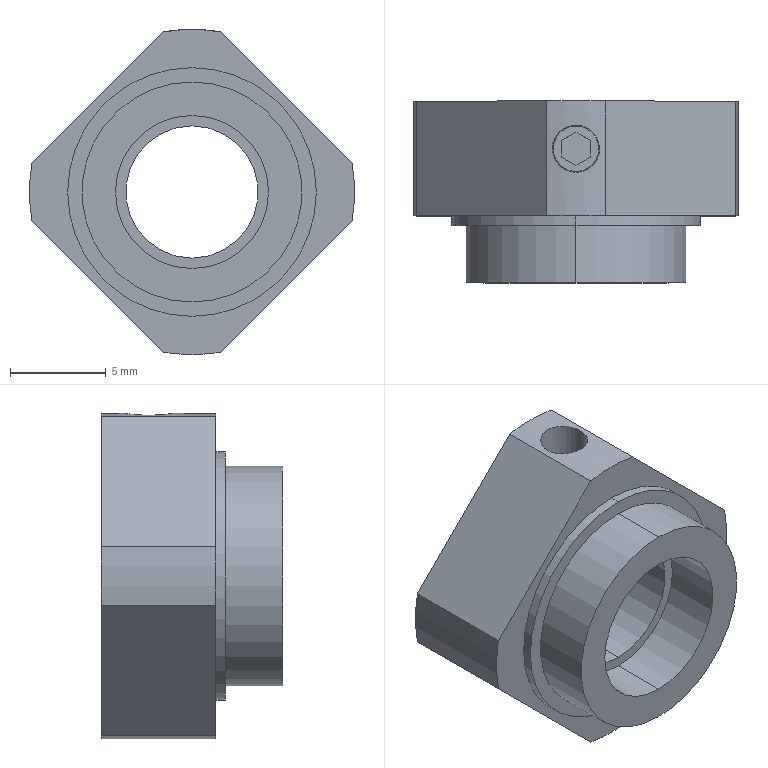Part | SolidWorks | features BaseBody 1 | 1 solid | 41 faces | box 17 x 9.5 x 17 mm | volume 1093 mm3 | plane 18 | cylinder 17 | cone 6 | commonest cylinder face diameters 17 x5 2.459 x4 6.917 x2 8 x2 11.5 x2 13 x2
STEP:
#1=CARTESIAN_POINT('',(290.547,1682.923,-1182.029));
#2=VERTEX_POINT('',#1);
#3=CARTESIAN_POINT('',(290.547,1682.923,-1175.111));
#4=VERTEX_POINT('',#3);
#5=CARTESIAN_POINT('',(290.547,1682.923,-1178.57));
#6=DIRECTION('',(0.,1.,0.));
#7=DIRECTION('',(0.,0.,-1.));
#8=AXIS2_PLACEMENT_3D('',#5,#6,#7);
#9=CIRCLE('',#8,3.459);
#10=EDGE_CURVE('',#2,#4,#9,.T.);
#11=ORIENTED_EDGE('',*,*,#10,.F.);
#12=CARTESIAN_POINT('',(290.547,1683.464,-1182.57));
#13=VERTEX_POINT('',#12);
#14=CARTESIAN_POINT('',(290.547,1683.464,-1182.57));
#15=DIRECTION('',(0.,0.7071,-0.7071));
#16=VECTOR('',#15,1000.);
#17=LINE('',#14,#16);
#18=EDGE_CURVE('',#2,#13,#17,.T.);
#19=ORIENTED_EDGE('',*,*,#18,.T.);
#20=CARTESIAN_POINT('',(290.547,1683.464,-1174.57));
#21=VERTEX_POINT('',#20);
#22=CARTESIAN_POINT('',(290.547,1683.464,-1178.57));
#23=DIRECTION('',(0.,-1.,0.));
#24=DIRECTION('',(0.,0.,1.));
#25=AXIS2_PLACEMENT_3D('',#22,#23,#24);
#26=CIRCLE('',#25,4.);
#27=EDGE_CURVE('',#21,#13,#26,.T.);
#28=ORIENTED_EDGE('',*,*,#27,.F.);
#29=CARTESIAN_POINT('',(290.547,1683.464,-1174.57));
#30=DIRECTION('',(0.,0.7071,0.7071));
#31=VECTOR('',#30,1000.);
#32=LINE('',#29,#31);
#33=EDGE_CURVE('',#4,#21,#32,.T.);
#34=ORIENTED_EDGE('',*,*,#33,.F.);
#35=EDGE_LOOP('',(#11,#19,#28,#34));
#36=FACE_OUTER_BOUND('',#35,.T.);
#37=CARTESIAN_POINT('',(290.547,1683.464,-1178.57));
#38=DIRECTION('',(0.,1.,0.));
#39=DIRECTION('',(0.,0.,1.));
#40=AXIS2_PLACEMENT_3D('',#37,#38,#39);
#41=CONICAL_SURFACE('',#40,4.,0.7854);
#42=ADVANCED_FACE('',(#36),#41,.F.);
#43=CARTESIAN_POINT('',(290.547,1683.464,-1187.07));
#44=VERTEX_POINT('',#43);
#45=CARTESIAN_POINT('',(289.006,1683.464,-1186.929));
#46=VERTEX_POINT('',#45);
#47=CARTESIAN_POINT('',(290.547,1683.464,-1178.57));
#48=DIRECTION('',(0.,1.,0.));
#49=DIRECTION('',(0.,0.,-1.));
#50=AXIS2_PLACEMENT_3D('',#47,#48,#49);
#51=CIRCLE('',#50,8.5);
#52=EDGE_CURVE('',#44,#46,#51,.T.);
#53=ORIENTED_EDGE('',*,*,#52,.F.);
#54=CARTESIAN_POINT('',(290.547,1677.464,-1187.07));
#55=VERTEX_POINT('',#54);
#56=CARTESIAN_POINT('',(290.547,1654.964,-1187.07));
#57=DIRECTION('',(0.,-1.,0.));
#58=VECTOR('',#57,1000.);
#59=LINE('',#56,#58);
#60=EDGE_CURVE('',#44,#55,#59,.T.);
#61=ORIENTED_EDGE('',*,*,#60,.T.);
#62=CARTESIAN_POINT('',(289.006,1677.464,-1186.929));
#63=VERTEX_POINT('',#62);
#64=CARTESIAN_POINT('',(290.547,1677.464,-1178.57));
#65=DIRECTION('',(0.,1.,0.));
#66=DIRECTION('',(0.,0.,-1.));
#67=AXIS2_PLACEMENT_3D('',#64,#65,#66);
#68=CIRCLE('',#67,8.5);
#69=EDGE_CURVE('',#55,#63,#68,.T.);
#70=ORIENTED_EDGE('',*,*,#69,.T.);
#71=CARTESIAN_POINT('',(289.006,1683.464,-1186.929));
#72=DIRECTION('',(0.,1.,0.));
#73=VECTOR('',#72,1000.);
#74=LINE('',#71,#73);
#75=EDGE_CURVE('',#63,#46,#74,.T.);
#76=ORIENTED_EDGE('',*,*,#75,.T.);
#77=EDGE_LOOP('',(#53,#61,#70,#76));
#78=FACE_OUTER_BOUND('',#77,.T.);
#79=CARTESIAN_POINT('',(290.547,1654.964,-1178.57));
#80=DIRECTION('',(0.,-1.,0.));
#81=DIRECTION('',(0.,0.,-1.));
#82=AXIS2_PLACEMENT_3D('',#79,#80,#81);
#83=CYLINDRICAL_SURFACE('',#82,8.5);
#84=ADVANCED_FACE('',(#78),#83,.T.);
#85=ORIENTED_EDGE('',*,*,#10,.T.);
#86=CARTESIAN_POINT('',(290.547,1682.194,-1175.111));
#87=VERTEX_POINT('',#86);
#88=CARTESIAN_POINT('',(290.547,1654.964,-1175.111));
#89=DIRECTION('',(0.,-1.,0.));
#90=VECTOR('',#89,1000.);
#91=LINE('',#88,#90);
#92=EDGE_CURVE('',#4,#87,#91,.T.);
#93=ORIENTED_EDGE('',*,*,#92,.T.);
#94=CARTESIAN_POINT('',(289.317,1680.964,-1175.337));
#95=VERTEX_POINT('',#94);
#96=CARTESIAN_POINT('',(289.317,1680.964,-1175.337));
#97=CARTESIAN_POINT('',(289.317,1681.128,-1175.337));
#98=CARTESIAN_POINT('',(289.35,1681.288,-1175.325));
#99=CARTESIAN_POINT('',(289.473,1681.585,-1175.282));
#100=CARTESIAN_POINT('',(289.565,1681.721,-1175.252));
#101=CARTESIAN_POINT('',(289.789,1681.945,-1175.193));
#102=CARTESIAN_POINT('',(289.925,1682.037,-1175.165));
#103=CARTESIAN_POINT('',(290.22,1682.16,-1175.124));
#104=CARTESIAN_POINT('',(290.383,1682.194,-1175.111));
#105=CARTESIAN_POINT('',(290.547,1682.194,-1175.111));
#106=B_SPLINE_CURVE_WITH_KNOTS('',3,(#96,#97,#98,#99,#100,#101,#102,#103,#104,#105),.UNSPECIFIED.,.F.,.F.,(4,2,2,2,4),(0.001937,0.002421,0.002905,0.003389,0.003874),.UNSPECIFIED.);
#107=EDGE_CURVE('',#95,#87,#106,.T.);
#108=ORIENTED_EDGE('',*,*,#107,.F.);
#109=CARTESIAN_POINT('',(290.547,1679.735,-1175.111));
#110=VERTEX_POINT('',#109);
#111=CARTESIAN_POINT('',(290.547,1679.735,-1175.111));
#112=CARTESIAN_POINT('',(290.383,1679.735,-1175.111));
#113=CARTESIAN_POINT('',(290.222,1679.767,-1175.123));
#114=CARTESIAN_POINT('',(289.925,1679.891,-1175.165));
#115=CARTESIAN_POINT('',(289.789,1679.982,-1175.193));
#116=CARTESIAN_POINT('',(289.565,1680.207,-1175.252));
#117=CARTESIAN_POINT('',(289.474,1680.343,-1175.282));
#118=CARTESIAN_POINT('',(289.35,1680.638,-1175.324));
#119=CARTESIAN_POINT('',(289.317,1680.8,-1175.337));
#120=CARTESIAN_POINT('',(289.317,1680.964,-1175.337));
#121=B_SPLINE_CURVE_WITH_KNOTS('',3,(#111,#112,#113,#114,#115,#116,#117,#118,#119,#120),.UNSPECIFIED.,.F.,.F.,(4,2,2,2,4),(0.000000144,0.0004843,0.0009685,0.001453,0.001937),.UNSPECIFIED.);
#122=EDGE_CURVE('',#110,#95,#121,.T.);
#123=ORIENTED_EDGE('',*,*,#122,.F.);
#124=CARTESIAN_POINT('',(290.547,1676.964,-1175.111));
#125=VERTEX_POINT('',#124);
#126=CARTESIAN_POINT('',(290.547,1654.964,-1175.111));
#127=DIRECTION('',(0.,-1.,0.));
#128=VECTOR('',#127,1000.);
#129=LINE('',#126,#128);
#130=EDGE_CURVE('',#110,#125,#129,.T.);
#131=ORIENTED_EDGE('',*,*,#130,.T.);
#132=CARTESIAN_POINT('',(290.547,1676.964,-1182.028));
#133=VERTEX_POINT('',#132);
#134=CARTESIAN_POINT('',(290.547,1676.964,-1178.57));
#135=DIRECTION('',(0.,1.,0.));
#136=DIRECTION('',(0.,0.,-1.));
#137=AXIS2_PLACEMENT_3D('',#134,#135,#136);
#138=CIRCLE('',#137,3.459);
#139=EDGE_CURVE('',#133,#125,#138,.T.);
#140=ORIENTED_EDGE('',*,*,#139,.F.);
#141=CARTESIAN_POINT('',(290.547,1654.964,-1182.028));
#142=DIRECTION('',(0.,-1.,0.));
#143=VECTOR('',#142,1000.);
#144=LINE('',#141,#143);
#145=EDGE_CURVE('',#2,#133,#144,.T.);
#146=ORIENTED_EDGE('',*,*,#145,.F.);
#147=EDGE_LOOP('',(#85,#93,#108,#123,#131,#140,#146));
#148=FACE_OUTER_BOUND('',#147,.T.);
#149=CARTESIAN_POINT('',(290.547,1654.964,-1178.57));
#150=DIRECTION('',(0.,-1.,0.));
#151=DIRECTION('',(0.,0.,-1.));
#152=AXIS2_PLACEMENT_3D('',#149,#150,#151);
#153=CYLINDRICAL_SURFACE('',#152,3.459);
#154=ADVANCED_FACE('',(#148),#153,.F.);
#155=CARTESIAN_POINT('',(289.317,1680.964,-1172.132));
#156=VERTEX_POINT('',#155);
#157=CARTESIAN_POINT('',(291.776,1680.964,-1172.132));
#158=VERTEX_POINT('',#157);
#159=CARTESIAN_POINT('',(290.547,1680.964,-1172.132));
#160=DIRECTION('',(0.,0.,1.));
#161=DIRECTION('',(1.,0.,0.));
#162=AXIS2_PLACEMENT_3D('',#159,#160,#161);
#163=CIRCLE('',#162,1.229);
#164=EDGE_CURVE('',#156,#158,#163,.T.);
#165=ORIENTED_EDGE('',*,*,#164,.F.);
#166=CARTESIAN_POINT('',(289.317,1680.964,-1170.159));
#167=VERTEX_POINT('',#166);
#168=CARTESIAN_POINT('',(289.317,1680.964,-1170.07));
#169=DIRECTION('',(0.,0.,1.));
#170=VECTOR('',#169,1000.);
#171=LINE('',#168,#170);
#172=EDGE_CURVE('',#156,#167,#171,.T.);
#173=ORIENTED_EDGE('',*,*,#172,.T.);
#174=CARTESIAN_POINT('',(291.776,1680.964,-1170.159));
#175=VERTEX_POINT('',#174);
#176=CARTESIAN_POINT('',(291.776,1680.964,-1170.159));
#177=CARTESIAN_POINT('',(291.776,1680.801,-1170.159));
#178=CARTESIAN_POINT('',(291.744,1680.642,-1170.155));
#179=CARTESIAN_POINT('',(291.621,1680.344,-1170.138));
#180=CARTESIAN_POINT('',(291.529,1680.208,-1170.126));
#181=CARTESIAN_POINT('',(291.303,1679.982,-1170.103));
#182=CARTESIAN_POINT('',(291.166,1679.89,-1170.091));
#183=CARTESIAN_POINT('',(290.871,1679.767,-1170.075));
#184=CARTESIAN_POINT('',(290.709,1679.735,-1170.07));
#185=CARTESIAN_POINT('',(290.384,1679.735,-1170.07));
#186=CARTESIAN_POINT('',(290.224,1679.767,-1170.075));
#187=CARTESIAN_POINT('',(289.927,1679.89,-1170.091));
#188=CARTESIAN_POINT('',(289.791,1679.981,-1170.103));
#189=CARTESIAN_POINT('',(289.564,1680.208,-1170.126));
#190=CARTESIAN_POINT('',(289.473,1680.344,-1170.138));
#191=CARTESIAN_POINT('',(289.35,1680.64,-1170.154));
#192=CARTESIAN_POINT('',(289.317,1680.801,-1170.159));
#193=CARTESIAN_POINT('',(289.317,1680.964,-1170.159));
#194=B_SPLINE_CURVE_WITH_KNOTS('',3,(#176,#177,#178,#179,#180,#181,#182,#183,#184,#185,#186,#187,#188,#189,#190,#191,#192,#193),.UNSPECIFIED.,.F.,.F.,(4,2,2,2,2,2,2,2,4),(-0.003846,-0.003366,-0.002885,-0.002404,-0.001923,-0.001442,-0.0009616,-0.0004808,0.),.UNSPECIFIED.);
#195=EDGE_CURVE('',#175,#167,#194,.T.);
#196=ORIENTED_EDGE('',*,*,#195,.F.);
#197=CARTESIAN_POINT('',(291.776,1680.964,-1170.07));
#198=DIRECTION('',(0.,0.,1.));
#199=VECTOR('',#198,1000.);
#200=LINE('',#197,#199);
#201=EDGE_CURVE('',#158,#175,#200,.T.);
#202=ORIENTED_EDGE('',*,*,#201,.F.);
#203=EDGE_LOOP('',(#165,#173,#196,#202));
#204=FACE_OUTER_BOUND('',#203,.T.);
#205=CARTESIAN_POINT('',(290.547,1680.964,-1170.07));
#206=DIRECTION('',(0.,0.,1.));
#207=DIRECTION('',(1.,0.,0.));
#208=AXIS2_PLACEMENT_3D('',#205,#206,#207);
#209=CYLINDRICAL_SURFACE('',#208,1.229);
#210=ADVANCED_FACE('',(#204),#209,.F.);
#211=CARTESIAN_POINT('',(291.776,1680.964,-1175.337));
#212=VERTEX_POINT('',#211);
#213=CARTESIAN_POINT('',(291.776,1680.964,-1175.337));
#214=CARTESIAN_POINT('',(291.776,1680.8,-1175.337));
#215=CARTESIAN_POINT('',(291.743,1680.64,-1175.325));
#216=CARTESIAN_POINT('',(291.62,1680.343,-1175.282));
#217=CARTESIAN_POINT('',(291.529,1680.207,-1175.252));
#218=CARTESIAN_POINT('',(291.304,1679.983,-1175.193));
#219=CARTESIAN_POINT('',(291.168,1679.891,-1175.165));
#220=CARTESIAN_POINT('',(290.873,1679.768,-1175.124));
#221=CARTESIAN_POINT('',(290.71,1679.735,-1175.111));
#222=CARTESIAN_POINT('',(290.547,1679.735,-1175.111));
#223=B_SPLINE_CURVE_WITH_KNOTS('',3,(#213,#214,#215,#216,#217,#218,#219,#220,#221,#222),.UNSPECIFIED.,.F.,.F.,(4,2,2,2,4),(-0.001937,-0.001452,-0.0009682,-0.000484,0.000000144),.UNSPECIFIED.);
#224=EDGE_CURVE('',#212,#110,#223,.T.);
#225=ORIENTED_EDGE('',*,*,#224,.T.);
#226=ORIENTED_EDGE('',*,*,#122,.T.);
#227=CARTESIAN_POINT('',(289.317,1680.964,-1174.882));
#228=VERTEX_POINT('',#227);
#229=CARTESIAN_POINT('',(289.317,1680.964,-1170.07));
#230=DIRECTION('',(0.,0.,1.));
#231=VECTOR('',#230,1000.);
#232=LINE('',#229,#231);
#233=EDGE_CURVE('',#95,#228,#232,.T.);
#234=ORIENTED_EDGE('',*,*,#233,.T.);
#235=CARTESIAN_POINT('',(291.776,1680.964,-1174.882));
#236=VERTEX_POINT('',#235);
#237=CARTESIAN_POINT('',(290.547,1680.964,-1174.882));
#238=DIRECTION('',(0.,0.,-1.));
#239=DIRECTION('',(1.,0.,0.));
#240=AXIS2_PLACEMENT_3D('',#237,#238,#239);
#241=CIRCLE('',#240,1.229);
#242=EDGE_CURVE('',#236,#228,#241,.T.);
#243=ORIENTED_EDGE('',*,*,#242,.F.);
#244=CARTESIAN_POINT('',(291.776,1680.964,-1170.07));
#245=DIRECTION('',(0.,0.,1.));
#246=VECTOR('',#245,1000.);
#247=LINE('',#244,#246);
#248=EDGE_CURVE('',#212,#236,#247,.T.);
#249=ORIENTED_EDGE('',*,*,#248,.F.);
#250=EDGE_LOOP('',(#225,#226,#234,#243,#249));
#251=FACE_OUTER_BOUND('',#250,.T.);
#252=CARTESIAN_POINT('',(290.547,1680.964,-1170.07));
#253=DIRECTION('',(0.,0.,1.));
#254=DIRECTION('',(1.,0.,0.));
#255=AXIS2_PLACEMENT_3D('',#252,#253,#254);
#256=CYLINDRICAL_SURFACE('',#255,1.229);
#257=ADVANCED_FACE('',(#251),#256,.F.);
#258=CARTESIAN_POINT('',(290.547,1677.464,-1172.07));
#259=VERTEX_POINT('',#258);
#260=CARTESIAN_POINT('',(290.547,1677.464,-1185.07));
#261=VERTEX_POINT('',#260);
#262=CARTESIAN_POINT('',(290.547,1677.464,-1178.57));
#263=DIRECTION('',(0.,1.,0.));
#264=DIRECTION('',(0.,0.,-1.));
#265=AXIS2_PLACEMENT_3D('',#262,#263,#264);
#266=CIRCLE('',#265,6.5);
#267=EDGE_CURVE('',#259,#261,#266,.T.);
#268=ORIENTED_EDGE('',*,*,#267,.F.);
#269=CARTESIAN_POINT('',(290.547,1676.964,-1172.07));
#270=VERTEX_POINT('',#269);
#271=CARTESIAN_POINT('',(290.547,1654.964,-1172.07));
#272=DIRECTION('',(0.,-1.,0.));
#273=VECTOR('',#272,1000.);
#274=LINE('',#271,#273);
#275=EDGE_CURVE('',#259,#270,#274,.T.);
#276=ORIENTED_EDGE('',*,*,#275,.T.);
#277=CARTESIAN_POINT('',(290.547,1676.964,-1185.07));
#278=VERTEX_POINT('',#277);
#279=CARTESIAN_POINT('',(290.547,1676.964,-1178.57));
#280=DIRECTION('',(0.,1.,0.));
#281=DIRECTION('',(0.,0.,-1.));
#282=AXIS2_PLACEMENT_3D('',#279,#280,#281);
#283=CIRCLE('',#282,6.5);
#284=EDGE_CURVE('',#270,#278,#283,.T.);
#285=ORIENTED_EDGE('',*,*,#284,.T.);
#286=CARTESIAN_POINT('',(290.547,1654.964,-1185.07));
#287=DIRECTION('',(0.,-1.,0.));
#288=VECTOR('',#287,1000.);
#289=LINE('',#286,#288);
#290=EDGE_CURVE('',#261,#278,#289,.T.);
#291=ORIENTED_EDGE('',*,*,#290,.F.);
#292=EDGE_LOOP('',(#268,#276,#285,#291));
#293=FACE_OUTER_BOUND('',#292,.T.);
#294=CARTESIAN_POINT('',(290.547,1654.964,-1178.57));
#295=DIRECTION('',(0.,-1.,0.));
#296=DIRECTION('',(0.,0.,-1.));
#297=AXIS2_PLACEMENT_3D('',#294,#295,#296);
#298=CYLINDRICAL_SURFACE('',#297,6.5);
#299=ADVANCED_FACE('',(#293),#298,.T.);
#300=CARTESIAN_POINT('',(289.353,1680.964,-1172.112));
#301=VERTEX_POINT('',#300);
#302=CARTESIAN_POINT('',(291.74,1680.964,-1172.112));
#303=VERTEX_POINT('',#302);
#304=CARTESIAN_POINT('',(290.547,1680.964,-1172.112));
#305=DIRECTION('',(0.,0.,-1.));
#306=DIRECTION('',(-1.,0.,0.));
#307=AXIS2_PLACEMENT_3D('',#304,#305,#306);
#308=CIRCLE('',#307,1.193);
#309=EDGE_CURVE('',#301,#303,#308,.T.);
#310=ORIENTED_EDGE('',*,*,#309,.T.);
#311=CARTESIAN_POINT('',(291.776,1680.964,-1172.132));
#312=DIRECTION('',(0.866,0.,-0.5));
#313=VECTOR('',#312,1000.);
#314=LINE('',#311,#313);
#315=EDGE_CURVE('',#303,#158,#314,.T.);
#316=ORIENTED_EDGE('',*,*,#315,.T.);
#317=CARTESIAN_POINT('',(290.547,1680.964,-1172.132));
#318=DIRECTION('',(0.,0.,1.));
#319=DIRECTION('',(1.,0.,0.));
#320=AXIS2_PLACEMENT_3D('',#317,#318,#319);
#321=CIRCLE('',#320,1.229);
#322=EDGE_CURVE('',#158,#156,#321,.T.);
#323=ORIENTED_EDGE('',*,*,#322,.T.);
#324=CARTESIAN_POINT('',(289.317,1680.964,-1172.132));
#325=DIRECTION('',(-0.866,0.,-0.5));
#326=VECTOR('',#325,1000.);
#327=LINE('',#324,#326);
#328=EDGE_CURVE('',#301,#156,#327,.T.);
#329=ORIENTED_EDGE('',*,*,#328,.F.);
#330=EDGE_LOOP('',(#310,#316,#323,#329));
#331=FACE_OUTER_BOUND('',#330,.T.);
#332=CARTESIAN_POINT('',(290.547,1680.964,-1172.132));
#333=DIRECTION('',(0.,0.,-1.));
#334=DIRECTION('',(-1.,0.,0.));
#335=AXIS2_PLACEMENT_3D('',#332,#333,#334);
#336=CONICAL_SURFACE('',#335,1.229,1.047);
#337=ADVANCED_FACE('',(#331),#336,.T.);
#338=CARTESIAN_POINT('',(291.547,1680.964,-1175.111));
#339=VERTEX_POINT('',#338);
#340=CARTESIAN_POINT('',(289.547,1680.964,-1175.111));
#341=VERTEX_POINT('',#340);
#342=CARTESIAN_POINT('',(290.547,1680.964,-1175.111));
#343=DIRECTION('',(0.,0.,1.));
#344=DIRECTION('',(1.,0.,0.));
#345=AXIS2_PLACEMENT_3D('',#342,#343,#344);
#346=CIRCLE('',#345,1.);
#347=EDGE_CURVE('',#339,#341,#346,.T.);
#348=ORIENTED_EDGE('',*,*,#347,.T.);
#349=CARTESIAN_POINT('',(289.317,1680.964,-1174.882));
#350=DIRECTION('',(-0.7071,0.,0.7071));
#351=VECTOR('',#350,1000.);
#352=LINE('',#349,#351);
#353=EDGE_CURVE('',#341,#228,#352,.T.);
#354=ORIENTED_EDGE('',*,*,#353,.T.);
#355=CARTESIAN_POINT('',(290.547,1680.964,-1174.882));
#356=DIRECTION('',(0.,0.,-1.));
#357=DIRECTION('',(1.,0.,0.));
#358=AXIS2_PLACEMENT_3D('',#355,#356,#357);
#359=CIRCLE('',#358,1.229);
#360=EDGE_CURVE('',#228,#236,#359,.T.);
#361=ORIENTED_EDGE('',*,*,#360,.T.);
#362=CARTESIAN_POINT('',(291.776,1680.964,-1174.882));
#363=DIRECTION('',(0.7071,0.,0.7071));
#364=VECTOR('',#363,1000.);
#365=LINE('',#362,#364);
#366=EDGE_CURVE('',#339,#236,#365,.T.);
#367=ORIENTED_EDGE('',*,*,#366,.F.);
#368=EDGE_LOOP('',(#348,#354,#361,#367));
#369=FACE_OUTER_BOUND('',#368,.T.);
#370=CARTESIAN_POINT('',(290.547,1680.964,-1174.882));
#371=DIRECTION('',(0.,0.,1.));
#372=DIRECTION('',(1.,0.,0.));
#373=AXIS2_PLACEMENT_3D('',#370,#371,#372);
#374=CONICAL_SURFACE('',#373,1.23,0.7854);
#375=ADVANCED_FACE('',(#369),#374,.T.);
#376=CARTESIAN_POINT('',(290.547,1676.964,-1174.57));
#377=VERTEX_POINT('',#376);
#378=CARTESIAN_POINT('',(290.547,1676.964,-1182.57));
#379=VERTEX_POINT('',#378);
#380=CARTESIAN_POINT('',(290.547,1676.964,-1178.57));
#381=DIRECTION('',(0.,-1.,0.));
#382=DIRECTION('',(0.,0.,-1.));
#383=AXIS2_PLACEMENT_3D('',#380,#381,#382);
#384=CIRCLE('',#383,4.);
#385=EDGE_CURVE('',#377,#379,#384,.T.);
#386=ORIENTED_EDGE('',*,*,#385,.F.);
#387=CARTESIAN_POINT('',(290.547,1673.964,-1174.57));
#388=VERTEX_POINT('',#387);
#389=CARTESIAN_POINT('',(290.547,1654.964,-1174.57));
#390=DIRECTION('',(0.,-1.,0.));
#391=VECTOR('',#390,1000.);
#392=LINE('',#389,#391);
#393=EDGE_CURVE('',#377,#388,#392,.T.);
#394=ORIENTED_EDGE('',*,*,#393,.T.);
#395=CARTESIAN_POINT('',(290.547,1673.964,-1182.57));
#396=VERTEX_POINT('',#395);
#397=CARTESIAN_POINT('',(290.547,1673.964,-1178.57));
#398=DIRECTION('',(0.,1.,0.));
#399=DIRECTION('',(0.,0.,-1.));
#400=AXIS2_PLACEMENT_3D('',#397,#398,#399);
#401=CIRCLE('',#400,4.);
#402=EDGE_CURVE('',#396,#388,#401,.T.);
#403=ORIENTED_EDGE('',*,*,#402,.F.);
#404=CARTESIAN_POINT('',(290.547,1654.964,-1182.57));
#405=DIRECTION('',(0.,-1.,0.));
#406=VECTOR('',#405,1000.);
#407=LINE('',#404,#406);
#408=EDGE_CURVE('',#379,#396,#407,.T.);
#409=ORIENTED_EDGE('',*,*,#408,.F.);
#410=EDGE_LOOP('',(#386,#394,#403,#409));
#411=FACE_OUTER_BOUND('',#410,.T.);
#412=CARTESIAN_POINT('',(290.547,1654.964,-1178.57));
#413=DIRECTION('',(0.,-1.,0.));
#414=DIRECTION('',(0.,0.,-1.));
#415=AXIS2_PLACEMENT_3D('',#412,#413,#414);
#416=CYLINDRICAL_SURFACE('',#415,4.);
#417=ADVANCED_FACE('',(#411),#416,.F.);
#418=CARTESIAN_POINT('',(290.547,1676.964,-1172.82));
#419=VERTEX_POINT('',#418);
#420=CARTESIAN_POINT('',(290.547,1676.964,-1184.32));
#421=VERTEX_POINT('',#420);
#422=CARTESIAN_POINT('',(290.547,1676.964,-1178.57));
#423=DIRECTION('',(0.,1.,0.));
#424=DIRECTION('',(0.,0.,-1.));
#425=AXIS2_PLACEMENT_3D('',#422,#423,#424);
#426=CIRCLE('',#425,5.75);
#427=EDGE_CURVE('',#419,#421,#426,.T.);
#428=ORIENTED_EDGE('',*,*,#427,.F.);
#429=CARTESIAN_POINT('',(290.547,1673.964,-1172.82));
#430=VERTEX_POINT('',#429);
#431=CARTESIAN_POINT('',(290.547,1654.964,-1172.82));
#432=DIRECTION('',(0.,-1.,0.));
#433=VECTOR('',#432,1000.);
#434=LINE('',#431,#433);
#435=EDGE_CURVE('',#419,#430,#434,.T.);
#436=ORIENTED_EDGE('',*,*,#435,.T.);
#437=CARTESIAN_POINT('',(290.547,1673.964,-1184.32));
#438=VERTEX_POINT('',#437);
#439=CARTESIAN_POINT('',(290.547,1673.964,-1178.57));
#440=DIRECTION('',(0.,-1.,0.));
#441=DIRECTION('',(0.,0.,-1.));
#442=AXIS2_PLACEMENT_3D('',#439,#440,#441);
#443=CIRCLE('',#442,5.75);
#444=EDGE_CURVE('',#438,#430,#443,.T.);
#445=ORIENTED_EDGE('',*,*,#444,.F.);
#446=CARTESIAN_POINT('',(290.547,1654.964,-1184.32));
#447=DIRECTION('',(0.,-1.,0.));
#448=VECTOR('',#447,1000.);
#449=LINE('',#446,#448);
#450=EDGE_CURVE('',#421,#438,#449,.T.);
#451=ORIENTED_EDGE('',*,*,#450,.F.);
#452=EDGE_LOOP('',(#428,#436,#445,#451));
#453=FACE_OUTER_BOUND('',#452,.T.);
#454=CARTESIAN_POINT('',(290.547,1654.964,-1178.57));
#455=DIRECTION('',(0.,-1.,0.));
#456=DIRECTION('',(0.,0.,-1.));
#457=AXIS2_PLACEMENT_3D('',#454,#455,#456);
#458=CYLINDRICAL_SURFACE('',#457,5.75);
#459=ADVANCED_FACE('',(#453),#458,.T.);
#460=ORIENTED_EDGE('',*,*,#27,.T.);
#461=CARTESIAN_POINT('',(290.547,1683.464,-1178.57));
#462=DIRECTION('',(0.,-1.,0.));
#463=DIRECTION('',(0.,0.,1.));
#464=AXIS2_PLACEMENT_3D('',#461,#462,#463);
#465=CIRCLE('',#464,4.);
#466=EDGE_CURVE('',#13,#21,#465,.T.);
#467=ORIENTED_EDGE('',*,*,#466,.T.);
#468=EDGE_LOOP('',(#460,#467));
#469=FACE_BOUND('',#468,.T.);
#470=CARTESIAN_POINT('',(298.906,1683.464,-1177.03));
#471=VERTEX_POINT('',#470);
#472=CARTESIAN_POINT('',(298.906,1683.464,-1180.11));
#473=VERTEX_POINT('',#472);
#474=CARTESIAN_POINT('',(290.547,1683.464,-1178.57));
#475=DIRECTION('',(0.,1.,0.));
#476=DIRECTION('',(0.,0.,-1.));
#477=AXIS2_PLACEMENT_3D('',#474,#475,#476);
#478=CIRCLE('',#477,8.5);
#479=EDGE_CURVE('',#471,#473,#478,.T.);
#480=ORIENTED_EDGE('',*,*,#479,.T.);
#481=CARTESIAN_POINT('',(292.087,1683.464,-1186.929));
#482=VERTEX_POINT('',#481);
#483=CARTESIAN_POINT('',(298.906,1683.464,-1180.11));
#484=DIRECTION('',(-0.7071,0.,-0.7071));
#485=VECTOR('',#484,1000.);
#486=LINE('',#483,#485);
#487=EDGE_CURVE('',#473,#482,#486,.T.);
#488=ORIENTED_EDGE('',*,*,#487,.T.);
#489=CARTESIAN_POINT('',(290.547,1683.464,-1178.57));
#490=DIRECTION('',(0.,1.,0.));
#491=DIRECTION('',(0.,0.,-1.));
#492=AXIS2_PLACEMENT_3D('',#489,#490,#491);
#493=CIRCLE('',#492,8.5);
#494=EDGE_CURVE('',#482,#44,#493,.T.);
#495=ORIENTED_EDGE('',*,*,#494,.T.);
#496=ORIENTED_EDGE('',*,*,#52,.T.);
#497=CARTESIAN_POINT('',(282.187,1683.464,-1180.11));
#498=VERTEX_POINT('',#497);
#499=CARTESIAN_POINT('',(289.006,1683.464,-1186.929));
#500=DIRECTION('',(-0.7071,0.,0.7071));
#501=VECTOR('',#500,1000.);
#502=LINE('',#499,#501);
#503=EDGE_CURVE('',#46,#498,#502,.T.);
#504=ORIENTED_EDGE('',*,*,#503,.T.);
#505=CARTESIAN_POINT('',(282.187,1683.464,-1177.03));
#506=VERTEX_POINT('',#505);
#507=CARTESIAN_POINT('',(290.547,1683.464,-1178.57));
#508=DIRECTION('',(0.,1.,0.));
#509=DIRECTION('',(0.,0.,-1.));
#510=AXIS2_PLACEMENT_3D('',#507,#508,#509);
#511=CIRCLE('',#510,8.5);
#512=EDGE_CURVE('',#498,#506,#511,.T.);
#513=ORIENTED_EDGE('',*,*,#512,.T.);
#514=CARTESIAN_POINT('',(289.006,1683.464,-1170.211));
#515=VERTEX_POINT('',#514);
#516=CARTESIAN_POINT('',(282.187,1683.464,-1177.03));
#517=DIRECTION('',(0.7071,0.,0.7071));
#518=VECTOR('',#517,1000.);
#519=LINE('',#516,#518);
#520=EDGE_CURVE('',#506,#515,#519,.T.);
#521=ORIENTED_EDGE('',*,*,#520,.T.);
#522=CARTESIAN_POINT('',(292.087,1683.464,-1170.211));
#523=VERTEX_POINT('',#522);
#524=CARTESIAN_POINT('',(290.547,1683.464,-1178.57));
#525=DIRECTION('',(0.,1.,0.));
#526=DIRECTION('',(0.,0.,-1.));
#527=AXIS2_PLACEMENT_3D('',#524,#525,#526);
#528=CIRCLE('',#527,8.5);
#529=EDGE_CURVE('',#515,#523,#528,.T.);
#530=ORIENTED_EDGE('',*,*,#529,.T.);
#531=CARTESIAN_POINT('',(292.087,1683.464,-1170.211));
#532=DIRECTION('',(0.7071,0.,-0.7071));
#533=VECTOR('',#532,1000.);
#534=LINE('',#531,#533);
#535=EDGE_CURVE('',#523,#471,#534,.T.);
#536=ORIENTED_EDGE('',*,*,#535,.T.);
#537=EDGE_LOOP('',(#480,#488,#495,#496,#504,#513,#521,#530,#536));
#538=FACE_OUTER_BOUND('',#537,.T.);
#539=CARTESIAN_POINT('',(290.547,1683.464,-1170.07));
#540=DIRECTION('',(0.,1.,0.));
#541=DIRECTION('',(0.,0.,1.));
#542=AXIS2_PLACEMENT_3D('',#539,#540,#541);
#543=PLANE('',#542);
#544=ADVANCED_FACE('',(#469,#538),#543,.T.);
#545=ORIENTED_EDGE('',*,*,#18,.F.);
#546=CARTESIAN_POINT('',(290.547,1682.923,-1178.57));
#547=DIRECTION('',(0.,1.,0.));
#548=DIRECTION('',(0.,0.,-1.));
#549=AXIS2_PLACEMENT_3D('',#546,#547,#548);
#550=CIRCLE('',#549,3.459);
#551=EDGE_CURVE('',#4,#2,#550,.T.);
#552=ORIENTED_EDGE('',*,*,#551,.F.);
#553=ORIENTED_EDGE('',*,*,#33,.T.);
#554=ORIENTED_EDGE('',*,*,#466,.F.);
#555=EDGE_LOOP('',(#545,#552,#553,#554));
#556=FACE_OUTER_BOUND('',#555,.T.);
#557=CARTESIAN_POINT('',(290.547,1683.464,-1178.57));
#558=DIRECTION('',(0.,1.,0.));
#559=DIRECTION('',(0.,0.,1.));
#560=AXIS2_PLACEMENT_3D('',#557,#558,#559);
#561=CONICAL_SURFACE('',#560,4.,0.7854);
#562=ADVANCED_FACE('',(#556),#561,.F.);
#563=ORIENTED_EDGE('',*,*,#487,.F.);
#564=CARTESIAN_POINT('',(298.906,1677.464,-1180.11));
#565=VERTEX_POINT('',#564);
#566=CARTESIAN_POINT('',(298.906,1683.464,-1180.11));
#567=DIRECTION('',(0.,1.,0.));
#568=VECTOR('',#567,1000.);
#569=LINE('',#566,#568);
#570=EDGE_CURVE('',#565,#473,#569,.T.);
#571=ORIENTED_EDGE('',*,*,#570,.F.);
#572=CARTESIAN_POINT('',(292.087,1677.464,-1186.929));
#573=VERTEX_POINT('',#572);
#574=CARTESIAN_POINT('',(292.087,1677.464,-1186.929));
#575=DIRECTION('',(0.7071,0.,0.7071));
#576=VECTOR('',#575,1000.);
#577=LINE('',#574,#576);
#578=EDGE_CURVE('',#573,#565,#577,.T.);
#579=ORIENTED_EDGE('',*,*,#578,.F.);
#580=CARTESIAN_POINT('',(292.087,1683.464,-1186.929));
#581=DIRECTION('',(0.,-1.,0.));
#582=VECTOR('',#581,1000.);
#583=LINE('',#580,#582);
#584=EDGE_CURVE('',#482,#573,#583,.T.);
#585=ORIENTED_EDGE('',*,*,#584,.F.);
#586=EDGE_LOOP('',(#563,#571,#579,#585));
#587=FACE_OUTER_BOUND('',#586,.T.);
#588=CARTESIAN_POINT('',(292.087,1683.464,-1186.929));
#589=DIRECTION('',(-0.7071,0.,0.7071));
#590=DIRECTION('',(0.7071,0.,0.7071));
#591=AXIS2_PLACEMENT_3D('',#588,#589,#590);
#592=PLANE('',#591);
#593=ADVANCED_FACE('',(#587),#592,.F.);
#594=CARTESIAN_POINT('',(298.906,1677.464,-1177.03));
#595=VERTEX_POINT('',#594);
#596=CARTESIAN_POINT('',(290.547,1677.464,-1178.57));
#597=DIRECTION('',(0.,1.,0.));
#598=DIRECTION('',(0.,0.,-1.));
#599=AXIS2_PLACEMENT_3D('',#596,#597,#598);
#600=CIRCLE('',#599,8.5);
#601=EDGE_CURVE('',#595,#565,#600,.T.);
#602=ORIENTED_EDGE('',*,*,#601,.T.);
#603=ORIENTED_EDGE('',*,*,#570,.T.);
#604=ORIENTED_EDGE('',*,*,#479,.F.);
#605=CARTESIAN_POINT('',(298.906,1654.964,-1177.03));
#606=DIRECTION('',(0.,-1.,0.));
#607=VECTOR('',#606,1000.);
#608=LINE('',#605,#607);
#609=EDGE_CURVE('',#471,#595,#608,.T.);
#610=ORIENTED_EDGE('',*,*,#609,.T.);
#611=EDGE_LOOP('',(#602,#603,#604,#610));
#612=FACE_OUTER_BOUND('',#611,.T.);
#613=CARTESIAN_POINT('',(290.547,1654.964,-1178.57));
#614=DIRECTION('',(0.,-1.,0.));
#615=DIRECTION('',(0.,0.,-1.));
#616=AXIS2_PLACEMENT_3D('',#613,#614,#615);
#617=CYLINDRICAL_SURFACE('',#616,8.5);
#618=ADVANCED_FACE('',(#612),#617,.T.);
#619=ORIENTED_EDGE('',*,*,#535,.F.);
#620=CARTESIAN_POINT('',(292.087,1677.464,-1170.211));
#621=VERTEX_POINT('',#620);
#622=CARTESIAN_POINT('',(292.087,1683.464,-1170.211));
#623=DIRECTION('',(0.,1.,0.));
#624=VECTOR('',#623,1000.);
#625=LINE('',#622,#624);
#626=EDGE_CURVE('',#621,#523,#625,.T.);
#627=ORIENTED_EDGE('',*,*,#626,.F.);
#628=CARTESIAN_POINT('',(292.087,1677.464,-1170.211));
#629=DIRECTION('',(-0.7071,0.,0.7071));
#630=VECTOR('',#629,1000.);
#631=LINE('',#628,#630);
#632=EDGE_CURVE('',#595,#621,#631,.T.);
#633=ORIENTED_EDGE('',*,*,#632,.F.);
#634=ORIENTED_EDGE('',*,*,#609,.F.);
#635=EDGE_LOOP('',(#619,#627,#633,#634));
#636=FACE_OUTER_BOUND('',#635,.T.);
#637=CARTESIAN_POINT('',(292.087,1683.464,-1170.211));
#638=DIRECTION('',(-0.7071,0.,-0.7071));
#639=DIRECTION('',(-0.7071,0.,0.7071));
#640=AXIS2_PLACEMENT_3D('',#637,#638,#639);
#641=PLANE('',#640);
#642=ADVANCED_FACE('',(#636),#641,.F.);
#643=ORIENTED_EDGE('',*,*,#195,.T.);
#644=CARTESIAN_POINT('',(289.317,1680.964,-1170.159));
#645=CARTESIAN_POINT('',(289.317,1681.127,-1170.159));
#646=CARTESIAN_POINT('',(289.349,1681.286,-1170.155));
#647=CARTESIAN_POINT('',(289.472,1681.584,-1170.138));
#648=CARTESIAN_POINT('',(289.564,1681.72,-1170.126));
#649=CARTESIAN_POINT('',(289.79,1681.946,-1170.103));
#650=CARTESIAN_POINT('',(289.927,1682.038,-1170.091));
#651=CARTESIAN_POINT('',(290.222,1682.161,-1170.075));
#652=CARTESIAN_POINT('',(290.384,1682.194,-1170.07));
#653=CARTESIAN_POINT('',(290.709,1682.194,-1170.07));
#654=CARTESIAN_POINT('',(290.869,1682.161,-1170.075));
#655=CARTESIAN_POINT('',(291.166,1682.038,-1170.091));
#656=CARTESIAN_POINT('',(291.302,1681.947,-1170.103));
#657=CARTESIAN_POINT('',(291.529,1681.721,-1170.126));
#658=CARTESIAN_POINT('',(291.62,1681.584,-1170.138));
#659=CARTESIAN_POINT('',(291.743,1681.288,-1170.154));
#660=CARTESIAN_POINT('',(291.776,1681.127,-1170.159));
#661=CARTESIAN_POINT('',(291.776,1680.964,-1170.159));
#662=B_SPLINE_CURVE_WITH_KNOTS('',3,(#644,#645,#646,#647,#648,#649,#650,#651,#652,#653,#654,#655,#656,#657,#658,#659,#660,#661),.UNSPECIFIED.,.F.,.F.,(4,2,2,2,2,2,2,2,4),(0.,0.0004808,0.0009616,0.001442,0.001923,0.002404,0.002885,0.003366,0.003846),.UNSPECIFIED.);
#663=EDGE_CURVE('',#167,#175,#662,.T.);
#664=ORIENTED_EDGE('',*,*,#663,.T.);
#665=EDGE_LOOP('',(#643,#664));
#666=FACE_BOUND('',#665,.T.);
#667=CARTESIAN_POINT('',(289.006,1677.464,-1170.211));
#668=VERTEX_POINT('',#667);
#669=CARTESIAN_POINT('',(290.547,1677.464,-1178.57));
#670=DIRECTION('',(0.,1.,0.));
#671=DIRECTION('',(0.,0.,-1.));
#672=AXIS2_PLACEMENT_3D('',#669,#670,#671);
#673=CIRCLE('',#672,8.5);
#674=EDGE_CURVE('',#668,#621,#673,.T.);
#675=ORIENTED_EDGE('',*,*,#674,.T.);
#676=ORIENTED_EDGE('',*,*,#626,.T.);
#677=ORIENTED_EDGE('',*,*,#529,.F.);
#678=CARTESIAN_POINT('',(289.006,1654.964,-1170.211));
#679=DIRECTION('',(0.,-1.,0.));
#680=VECTOR('',#679,1000.);
#681=LINE('',#678,#680);
#682=EDGE_CURVE('',#515,#668,#681,.T.);
#683=ORIENTED_EDGE('',*,*,#682,.T.);
#684=EDGE_LOOP('',(#675,#676,#677,#683));
#685=FACE_OUTER_BOUND('',#684,.T.);
#686=CARTESIAN_POINT('',(290.547,1654.964,-1178.57));
#687=DIRECTION('',(0.,-1.,0.));
#688=DIRECTION('',(0.,0.,-1.));
#689=AXIS2_PLACEMENT_3D('',#686,#687,#688);
#690=CYLINDRICAL_SURFACE('',#689,8.5);
#691=ADVANCED_FACE('',(#666,#685),#690,.T.);
#692=ORIENTED_EDGE('',*,*,#520,.F.);
#693=CARTESIAN_POINT('',(282.187,1677.464,-1177.03));
#694=VERTEX_POINT('',#693);
#695=CARTESIAN_POINT('',(282.187,1683.464,-1177.03));
#696=DIRECTION('',(0.,1.,0.));
#697=VECTOR('',#696,1000.);
#698=LINE('',#695,#697);
#699=EDGE_CURVE('',#694,#506,#698,.T.);
#700=ORIENTED_EDGE('',*,*,#699,.F.);
#701=CARTESIAN_POINT('',(282.187,1677.464,-1177.03));
#702=DIRECTION('',(-0.7071,0.,-0.7071));
#703=VECTOR('',#702,1000.);
#704=LINE('',#701,#703);
#705=EDGE_CURVE('',#668,#694,#704,.T.);
#706=ORIENTED_EDGE('',*,*,#705,.F.);
#707=ORIENTED_EDGE('',*,*,#682,.F.);
#708=EDGE_LOOP('',(#692,#700,#706,#707));
#709=FACE_OUTER_BOUND('',#708,.T.);
#710=CARTESIAN_POINT('',(282.187,1683.464,-1177.03));
#711=DIRECTION('',(0.7071,0.,-0.7071));
#712=DIRECTION('',(-0.7071,0.,-0.7071));
#713=AXIS2_PLACEMENT_3D('',#710,#711,#712);
#714=PLANE('',#713);
#715=ADVANCED_FACE('',(#709),#714,.F.);
#716=ORIENTED_EDGE('',*,*,#512,.F.);
#717=CARTESIAN_POINT('',(282.187,1677.464,-1180.11));
#718=VERTEX_POINT('',#717);
#719=CARTESIAN_POINT('',(282.187,1654.964,-1180.11));
#720=DIRECTION('',(0.,-1.,0.));
#721=VECTOR('',#720,1000.);
#722=LINE('',#719,#721);
#723=EDGE_CURVE('',#498,#718,#722,.T.);
#724=ORIENTED_EDGE('',*,*,#723,.T.);
#725=CARTESIAN_POINT('',(290.547,1677.464,-1178.57));
#726=DIRECTION('',(0.,1.,0.));
#727=DIRECTION('',(0.,0.,-1.));
#728=AXIS2_PLACEMENT_3D('',#725,#726,#727);
#729=CIRCLE('',#728,8.5);
#730=EDGE_CURVE('',#718,#694,#729,.T.);
#731=ORIENTED_EDGE('',*,*,#730,.T.);
#732=ORIENTED_EDGE('',*,*,#699,.T.);
#733=EDGE_LOOP('',(#716,#724,#731,#732));
#734=FACE_OUTER_BOUND('',#733,.T.);
#735=CARTESIAN_POINT('',(290.547,1654.964,-1178.57));
#736=DIRECTION('',(0.,-1.,0.));
#737=DIRECTION('',(0.,0.,-1.));
#738=AXIS2_PLACEMENT_3D('',#735,#736,#737);
#739=CYLINDRICAL_SURFACE('',#738,8.5);
#740=ADVANCED_FACE('',(#734),#739,.T.);
#741=ORIENTED_EDGE('',*,*,#503,.F.);
#742=ORIENTED_EDGE('',*,*,#75,.F.);
#743=CARTESIAN_POINT('',(282.187,1677.464,-1180.11));
#744=DIRECTION('',(0.7071,0.,-0.7071));
#745=VECTOR('',#744,1000.);
#746=LINE('',#743,#745);
#747=EDGE_CURVE('',#718,#63,#746,.T.);
#748=ORIENTED_EDGE('',*,*,#747,.F.);
#749=ORIENTED_EDGE('',*,*,#723,.F.);
#750=EDGE_LOOP('',(#741,#742,#748,#749));
#751=FACE_OUTER_BOUND('',#750,.T.);
#752=CARTESIAN_POINT('',(282.187,1683.464,-1180.11));
#753=DIRECTION('',(0.7071,0.,0.7071));
#754=DIRECTION('',(0.7071,0.,-0.7071));
#755=AXIS2_PLACEMENT_3D('',#752,#753,#754);
#756=PLANE('',#755);
#757=ADVANCED_FACE('',(#751),#756,.F.);
#758=ORIENTED_EDGE('',*,*,#60,.F.);
#759=ORIENTED_EDGE('',*,*,#494,.F.);
#760=ORIENTED_EDGE('',*,*,#584,.T.);
#761=CARTESIAN_POINT('',(290.547,1677.464,-1178.57));
#762=DIRECTION('',(0.,1.,0.));
#763=DIRECTION('',(0.,0.,-1.));
#764=AXIS2_PLACEMENT_3D('',#761,#762,#763);
#765=CIRCLE('',#764,8.5);
#766=EDGE_CURVE('',#573,#55,#765,.T.);
#767=ORIENTED_EDGE('',*,*,#766,.T.);
#768=EDGE_LOOP('',(#758,#759,#760,#767));
#769=FACE_OUTER_BOUND('',#768,.T.);
#770=CARTESIAN_POINT('',(290.547,1654.964,-1178.57));
#771=DIRECTION('',(0.,-1.,0.));
#772=DIRECTION('',(0.,0.,-1.));
#773=AXIS2_PLACEMENT_3D('',#770,#771,#772);
#774=CYLINDRICAL_SURFACE('',#773,8.5);
#775=ADVANCED_FACE('',(#769),#774,.T.);
#776=ORIENTED_EDGE('',*,*,#92,.F.);
#777=ORIENTED_EDGE('',*,*,#551,.T.);
#778=ORIENTED_EDGE('',*,*,#145,.T.);
#779=CARTESIAN_POINT('',(290.547,1676.964,-1178.57));
#780=DIRECTION('',(0.,1.,0.));
#781=DIRECTION('',(0.,0.,-1.));
#782=AXIS2_PLACEMENT_3D('',#779,#780,#781);
#783=CIRCLE('',#782,3.459);
#784=EDGE_CURVE('',#125,#133,#783,.T.);
#785=ORIENTED_EDGE('',*,*,#784,.F.);
#786=ORIENTED_EDGE('',*,*,#130,.F.);
#787=ORIENTED_EDGE('',*,*,#224,.F.);
#788=CARTESIAN_POINT('',(290.547,1682.194,-1175.111));
#789=CARTESIAN_POINT('',(290.71,1682.194,-1175.111));
#790=CARTESIAN_POINT('',(290.871,1682.161,-1175.123));
#791=CARTESIAN_POINT('',(291.168,1682.037,-1175.165));
#792=CARTESIAN_POINT('',(291.304,1681.946,-1175.193));
#793=CARTESIAN_POINT('',(291.528,1681.721,-1175.252));
#794=CARTESIAN_POINT('',(291.62,1681.585,-1175.282));
#795=CARTESIAN_POINT('',(291.743,1681.29,-1175.324));
#796=CARTESIAN_POINT('',(291.776,1681.128,-1175.337));
#797=CARTESIAN_POINT('',(291.776,1680.964,-1175.337));
#798=B_SPLINE_CURVE_WITH_KNOTS('',3,(#788,#789,#790,#791,#792,#793,#794,#795,#796,#797),.UNSPECIFIED.,.F.,.F.,(4,2,2,2,4),(0.003874,0.004358,0.004842,0.005326,0.00581),.UNSPECIFIED.);
#799=EDGE_CURVE('',#87,#212,#798,.T.);
#800=ORIENTED_EDGE('',*,*,#799,.F.);
#801=EDGE_LOOP('',(#776,#777,#778,#785,#786,#787,#800));
#802=FACE_OUTER_BOUND('',#801,.T.);
#803=CARTESIAN_POINT('',(290.547,1654.964,-1178.57));
#804=DIRECTION('',(0.,-1.,0.));
#805=DIRECTION('',(0.,0.,-1.));
#806=AXIS2_PLACEMENT_3D('',#803,#804,#805);
#807=CYLINDRICAL_SURFACE('',#806,3.459);
#808=ADVANCED_FACE('',(#802),#807,.F.);
#809=CARTESIAN_POINT('',(290.547,1677.464,-1178.57));
#810=DIRECTION('',(0.,1.,0.));
#811=DIRECTION('',(0.,0.,-1.));
#812=AXIS2_PLACEMENT_3D('',#809,#810,#811);
#813=CIRCLE('',#812,6.5);
#814=EDGE_CURVE('',#261,#259,#813,.T.);
#815=ORIENTED_EDGE('',*,*,#814,.T.);
#816=ORIENTED_EDGE('',*,*,#267,.T.);
#817=EDGE_LOOP('',(#815,#816));
#818=FACE_BOUND('',#817,.T.);
#819=ORIENTED_EDGE('',*,*,#766,.F.);
#820=ORIENTED_EDGE('',*,*,#578,.T.);
#821=ORIENTED_EDGE('',*,*,#601,.F.);
#822=ORIENTED_EDGE('',*,*,#632,.T.);
#823=ORIENTED_EDGE('',*,*,#674,.F.);
#824=ORIENTED_EDGE('',*,*,#705,.T.);
#825=ORIENTED_EDGE('',*,*,#730,.F.);
#826=ORIENTED_EDGE('',*,*,#747,.T.);
#827=ORIENTED_EDGE('',*,*,#69,.F.);
#828=EDGE_LOOP('',(#819,#820,#821,#822,#823,#824,#825,#826,#827));
#829=FACE_OUTER_BOUND('',#828,.T.);
#830=CARTESIAN_POINT('',(290.547,1677.464,-1172.07));
#831=DIRECTION('',(0.,-1.,0.));
#832=DIRECTION('',(0.,0.,-1.));
#833=AXIS2_PLACEMENT_3D('',#830,#831,#832);
#834=PLANE('',#833);
#835=ADVANCED_FACE('',(#818,#829),#834,.T.);
#836=ORIENTED_EDGE('',*,*,#172,.F.);
#837=ORIENTED_EDGE('',*,*,#322,.F.);
#838=ORIENTED_EDGE('',*,*,#201,.T.);
#839=ORIENTED_EDGE('',*,*,#663,.F.);
#840=EDGE_LOOP('',(#836,#837,#838,#839));
#841=FACE_OUTER_BOUND('',#840,.T.);
#842=CARTESIAN_POINT('',(290.547,1680.964,-1170.07));
#843=DIRECTION('',(0.,0.,1.));
#844=DIRECTION('',(1.,0.,0.));
#845=AXIS2_PLACEMENT_3D('',#842,#843,#844);
#846=CYLINDRICAL_SURFACE('',#845,1.229);
#847=ADVANCED_FACE('',(#841),#846,.F.);
#848=ORIENTED_EDGE('',*,*,#233,.F.);
#849=ORIENTED_EDGE('',*,*,#107,.T.);
#850=ORIENTED_EDGE('',*,*,#799,.T.);
#851=ORIENTED_EDGE('',*,*,#248,.T.);
#852=ORIENTED_EDGE('',*,*,#360,.F.);
#853=EDGE_LOOP('',(#848,#849,#850,#851,#852));
#854=FACE_OUTER_BOUND('',#853,.T.);
#855=CARTESIAN_POINT('',(290.547,1680.964,-1170.07));
#856=DIRECTION('',(0.,0.,1.));
#857=DIRECTION('',(1.,0.,0.));
#858=AXIS2_PLACEMENT_3D('',#855,#856,#857);
#859=CYLINDRICAL_SURFACE('',#858,1.229);
#860=ADVANCED_FACE('',(#854),#859,.F.);
#861=ORIENTED_EDGE('',*,*,#139,.T.);
#862=ORIENTED_EDGE('',*,*,#784,.T.);
#863=EDGE_LOOP('',(#861,#862));
#864=FACE_BOUND('',#863,.T.);
#865=CARTESIAN_POINT('',(290.547,1676.964,-1178.57));
#866=DIRECTION('',(0.,-1.,0.));
#867=DIRECTION('',(0.,0.,-1.));
#868=AXIS2_PLACEMENT_3D('',#865,#866,#867);
#869=CIRCLE('',#868,4.);
#870=EDGE_CURVE('',#379,#377,#869,.T.);
#871=ORIENTED_EDGE('',*,*,#870,.T.);
#872=ORIENTED_EDGE('',*,*,#385,.T.);
#873=EDGE_LOOP('',(#871,#872));
#874=FACE_OUTER_BOUND('',#873,.T.);
#875=CARTESIAN_POINT('',(290.547,1676.964,-1174.57));
#876=DIRECTION('',(0.,-1.,0.));
#877=DIRECTION('',(0.,0.,-1.));
#878=AXIS2_PLACEMENT_3D('',#875,#876,#877);
#879=PLANE('',#878);
#880=ADVANCED_FACE('',(#864,#874),#879,.T.);
#881=ORIENTED_EDGE('',*,*,#275,.F.);
#882=ORIENTED_EDGE('',*,*,#814,.F.);
#883=ORIENTED_EDGE('',*,*,#290,.T.);
#884=CARTESIAN_POINT('',(290.547,1676.964,-1178.57));
#885=DIRECTION('',(0.,1.,0.));
#886=DIRECTION('',(0.,0.,-1.));
#887=AXIS2_PLACEMENT_3D('',#884,#885,#886);
#888=CIRCLE('',#887,6.5);
#889=EDGE_CURVE('',#278,#270,#888,.T.);
#890=ORIENTED_EDGE('',*,*,#889,.T.);
#891=EDGE_LOOP('',(#881,#882,#883,#890));
#892=FACE_OUTER_BOUND('',#891,.T.);
#893=CARTESIAN_POINT('',(290.547,1654.964,-1178.57));
#894=DIRECTION('',(0.,-1.,0.));
#895=DIRECTION('',(0.,0.,-1.));
#896=AXIS2_PLACEMENT_3D('',#893,#894,#895);
#897=CYLINDRICAL_SURFACE('',#896,6.5);
#898=ADVANCED_FACE('',(#892),#897,.T.);
#899=ORIENTED_EDGE('',*,*,#315,.F.);
#900=CARTESIAN_POINT('',(290.547,1680.964,-1172.112));
#901=DIRECTION('',(0.,0.,-1.));
#902=DIRECTION('',(-1.,0.,0.));
#903=AXIS2_PLACEMENT_3D('',#900,#901,#902);
#904=CIRCLE('',#903,1.193);
#905=EDGE_CURVE('',#303,#301,#904,.T.);
#906=ORIENTED_EDGE('',*,*,#905,.T.);
#907=ORIENTED_EDGE('',*,*,#328,.T.);
#908=ORIENTED_EDGE('',*,*,#164,.T.);
#909=EDGE_LOOP('',(#899,#906,#907,#908));
#910=FACE_OUTER_BOUND('',#909,.T.);
#911=CARTESIAN_POINT('',(290.547,1680.964,-1172.132));
#912=DIRECTION('',(0.,0.,-1.));
#913=DIRECTION('',(-1.,0.,0.));
#914=AXIS2_PLACEMENT_3D('',#911,#912,#913);
#915=CONICAL_SURFACE('',#914,1.229,1.047);
#916=ADVANCED_FACE('',(#910),#915,.T.);
#917=ORIENTED_EDGE('',*,*,#353,.F.);
#918=CARTESIAN_POINT('',(290.547,1680.964,-1175.111));
#919=DIRECTION('',(0.,0.,1.));
#920=DIRECTION('',(1.,0.,0.));
#921=AXIS2_PLACEMENT_3D('',#918,#919,#920);
#922=CIRCLE('',#921,1.);
#923=EDGE_CURVE('',#341,#339,#922,.T.);
#924=ORIENTED_EDGE('',*,*,#923,.T.);
#925=ORIENTED_EDGE('',*,*,#366,.T.);
#926=ORIENTED_EDGE('',*,*,#242,.T.);
#927=EDGE_LOOP('',(#917,#924,#925,#926));
#928=FACE_OUTER_BOUND('',#927,.T.);
#929=CARTESIAN_POINT('',(290.547,1680.964,-1174.882));
#930=DIRECTION('',(0.,0.,1.));
#931=DIRECTION('',(1.,0.,0.));
#932=AXIS2_PLACEMENT_3D('',#929,#930,#931);
#933=CONICAL_SURFACE('',#932,1.23,0.7854);
#934=ADVANCED_FACE('',(#928),#933,.T.);
#935=ORIENTED_EDGE('',*,*,#393,.F.);
#936=ORIENTED_EDGE('',*,*,#870,.F.);
#937=ORIENTED_EDGE('',*,*,#408,.T.);
#938=CARTESIAN_POINT('',(290.547,1673.964,-1178.57));
#939=DIRECTION('',(0.,1.,0.));
#940=DIRECTION('',(0.,0.,-1.));
#941=AXIS2_PLACEMENT_3D('',#938,#939,#940);
#942=CIRCLE('',#941,4.);
#943=EDGE_CURVE('',#388,#396,#942,.T.);
#944=ORIENTED_EDGE('',*,*,#943,.F.);
#945=EDGE_LOOP('',(#935,#936,#937,#944));
#946=FACE_OUTER_BOUND('',#945,.T.);
#947=CARTESIAN_POINT('',(290.547,1654.964,-1178.57));
#948=DIRECTION('',(0.,-1.,0.));
#949=DIRECTION('',(0.,0.,-1.));
#950=AXIS2_PLACEMENT_3D('',#947,#948,#949);
#951=CYLINDRICAL_SURFACE('',#950,4.);
#952=ADVANCED_FACE('',(#946),#951,.F.);
#953=CARTESIAN_POINT('',(290.547,1676.964,-1178.57));
#954=DIRECTION('',(0.,1.,0.));
#955=DIRECTION('',(0.,0.,-1.));
#956=AXIS2_PLACEMENT_3D('',#953,#954,#955);
#957=CIRCLE('',#956,5.75);
#958=EDGE_CURVE('',#421,#419,#957,.T.);
#959=ORIENTED_EDGE('',*,*,#958,.T.);
#960=ORIENTED_EDGE('',*,*,#427,.T.);
#961=EDGE_LOOP('',(#959,#960));
#962=FACE_BOUND('',#961,.T.);
#963=ORIENTED_EDGE('',*,*,#889,.F.);
#964=ORIENTED_EDGE('',*,*,#284,.F.);
#965=EDGE_LOOP('',(#963,#964));
#966=FACE_OUTER_BOUND('',#965,.T.);
#967=CARTESIAN_POINT('',(290.547,1676.964,-1172.82));
#968=DIRECTION('',(0.,-1.,0.));
#969=DIRECTION('',(0.,0.,-1.));
#970=AXIS2_PLACEMENT_3D('',#967,#968,#969);
#971=PLANE('',#970);
#972=ADVANCED_FACE('',(#962,#966),#971,.T.);
#973=CARTESIAN_POINT('',(291.297,1680.531,-1172.111));
#974=VERTEX_POINT('',#973);
#975=CARTESIAN_POINT('',(290.547,1680.098,-1172.111));
#976=VERTEX_POINT('',#975);
#977=CARTESIAN_POINT('',(291.297,1680.531,-1172.111));
#978=DIRECTION('',(-0.866,-0.5,0.));
#979=VECTOR('',#978,1000.);
#980=LINE('',#977,#979);
#981=EDGE_CURVE('',#974,#976,#980,.T.);
#982=ORIENTED_EDGE('',*,*,#981,.T.);
#983=CARTESIAN_POINT('',(289.797,1680.531,-1172.111));
#984=VERTEX_POINT('',#983);
#985=CARTESIAN_POINT('',(290.547,1680.098,-1172.111));
#986=DIRECTION('',(-0.866,0.5,0.));
#987=VECTOR('',#986,1000.);
#988=LINE('',#985,#987);
#989=EDGE_CURVE('',#976,#984,#988,.T.);
#990=ORIENTED_EDGE('',*,*,#989,.T.);
#991=CARTESIAN_POINT('',(289.797,1681.397,-1172.111));
#992=VERTEX_POINT('',#991);
#993=CARTESIAN_POINT('',(289.797,1682.158,-1172.111));
#994=DIRECTION('',(0.,1.,0.));
#995=VECTOR('',#994,1000.);
#996=LINE('',#993,#995);
#997=EDGE_CURVE('',#984,#992,#996,.T.);
#998=ORIENTED_EDGE('',*,*,#997,.T.);
#999=CARTESIAN_POINT('',(290.547,1681.83,-1172.111));
#1000=VERTEX_POINT('',#999);
#1001=CARTESIAN_POINT('',(289.797,1681.397,-1172.111));
#1002=DIRECTION('',(0.866,0.5,0.));
#1003=VECTOR('',#1002,1000.);
#1004=LINE('',#1001,#1003);
#1005=EDGE_CURVE('',#992,#1000,#1004,.T.);
#1006=ORIENTED_EDGE('',*,*,#1005,.T.);
#1007=CARTESIAN_POINT('',(291.297,1681.397,-1172.111));
#1008=VERTEX_POINT('',#1007);
#1009=CARTESIAN_POINT('',(290.547,1681.83,-1172.111));
#1010=DIRECTION('',(0.866,-0.5,0.));
#1011=VECTOR('',#1010,1000.);
#1012=LINE('',#1009,#1011);
#1013=EDGE_CURVE('',#1000,#1008,#1012,.T.);
#1014=ORIENTED_EDGE('',*,*,#1013,.T.);
#1015=CARTESIAN_POINT('',(291.297,1682.158,-1172.111));
#1016=DIRECTION('',(0.,-1.,0.));
#1017=VECTOR('',#1016,1000.);
#1018=LINE('',#1015,#1017);
#1019=EDGE_CURVE('',#1008,#974,#1018,.T.);
#1020=ORIENTED_EDGE('',*,*,#1019,.T.);
#1021=EDGE_LOOP('',(#982,#990,#998,#1006,#1014,#1020));
#1022=FACE_BOUND('',#1021,.T.);
#1023=ORIENTED_EDGE('',*,*,#309,.F.);
#1024=ORIENTED_EDGE('',*,*,#905,.F.);
#1025=EDGE_LOOP('',(#1023,#1024));
#1026=FACE_OUTER_BOUND('',#1025,.T.);
#1027=CARTESIAN_POINT('',(290.547,1682.158,-1172.111));
#1028=DIRECTION('',(0.,0.,1.));
#1029=DIRECTION('',(1.,0.,0.));
#1030=AXIS2_PLACEMENT_3D('',#1027,#1028,#1029);
#1031=PLANE('',#1030);
#1032=ADVANCED_FACE('',(#1022,#1026),#1031,.T.);
#1033=ORIENTED_EDGE('',*,*,#347,.F.);
#1034=ORIENTED_EDGE('',*,*,#923,.F.);
#1035=EDGE_LOOP('',(#1033,#1034));
#1036=FACE_OUTER_BOUND('',#1035,.T.);
#1037=CARTESIAN_POINT('',(290.547,1681.964,-1175.111));
#1038=DIRECTION('',(0.,0.,-1.));
#1039=DIRECTION('',(-1.,0.,0.));
#1040=AXIS2_PLACEMENT_3D('',#1037,#1038,#1039);
#1041=PLANE('',#1040);
#1042=ADVANCED_FACE('',(#1036),#1041,.T.);
#1043=ORIENTED_EDGE('',*,*,#402,.T.);
#1044=ORIENTED_EDGE('',*,*,#943,.T.);
#1045=EDGE_LOOP('',(#1043,#1044));
#1046=FACE_BOUND('',#1045,.T.);
#1047=ORIENTED_EDGE('',*,*,#444,.T.);
#1048=CARTESIAN_POINT('',(290.547,1673.964,-1178.57));
#1049=DIRECTION('',(0.,-1.,0.));
#1050=DIRECTION('',(0.,0.,-1.));
#1051=AXIS2_PLACEMENT_3D('',#1048,#1049,#1050);
#1052=CIRCLE('',#1051,5.75);
#1053=EDGE_CURVE('',#430,#438,#1052,.T.);
#1054=ORIENTED_EDGE('',*,*,#1053,.T.);
#1055=EDGE_LOOP('',(#1047,#1054));
#1056=FACE_OUTER_BOUND('',#1055,.T.);
#1057=CARTESIAN_POINT('',(290.547,1673.964,-1172.82));
#1058=DIRECTION('',(0.,-1.,0.));
#1059=DIRECTION('',(0.,0.,-1.));
#1060=AXIS2_PLACEMENT_3D('',#1057,#1058,#1059);
#1061=PLANE('',#1060);
#1062=ADVANCED_FACE('',(#1046,#1056),#1061,.T.);
#1063=ORIENTED_EDGE('',*,*,#435,.F.);
#1064=ORIENTED_EDGE('',*,*,#958,.F.);
#1065=ORIENTED_EDGE('',*,*,#450,.T.);
#1066=ORIENTED_EDGE('',*,*,#1053,.F.);
#1067=EDGE_LOOP('',(#1063,#1064,#1065,#1066));
#1068=FACE_OUTER_BOUND('',#1067,.T.);
#1069=CARTESIAN_POINT('',(290.547,1654.964,-1178.57));
#1070=DIRECTION('',(0.,-1.,0.));
#1071=DIRECTION('',(0.,0.,-1.));
#1072=AXIS2_PLACEMENT_3D('',#1069,#1070,#1071);
#1073=CYLINDRICAL_SURFACE('',#1072,5.75);
#1074=ADVANCED_FACE('',(#1068),#1073,.T.);
#1075=CARTESIAN_POINT('',(289.797,1680.531,-1173.312));
#1076=VERTEX_POINT('',#1075);
#1077=CARTESIAN_POINT('',(290.547,1680.098,-1173.312));
#1078=VERTEX_POINT('',#1077);
#1079=CARTESIAN_POINT('',(289.797,1680.531,-1173.312));
#1080=DIRECTION('',(0.866,-0.5,0.));
#1081=VECTOR('',#1080,1000.);
#1082=LINE('',#1079,#1081);
#1083=EDGE_CURVE('',#1076,#1078,#1082,.T.);
#1084=ORIENTED_EDGE('',*,*,#1083,.F.);
#1085=CARTESIAN_POINT('',(289.797,1680.531,-1173.312));
#1086=DIRECTION('',(0.,0.,-1.));
#1087=VECTOR('',#1086,1000.);
#1088=LINE('',#1085,#1087);
#1089=EDGE_CURVE('',#984,#1076,#1088,.T.);
#1090=ORIENTED_EDGE('',*,*,#1089,.F.);
#1091=ORIENTED_EDGE('',*,*,#989,.F.);
#1092=CARTESIAN_POINT('',(290.547,1680.098,-1173.312));
#1093=DIRECTION('',(0.,0.,1.));
#1094=VECTOR('',#1093,1000.);
#1095=LINE('',#1092,#1094);
#1096=EDGE_CURVE('',#1078,#976,#1095,.T.);
#1097=ORIENTED_EDGE('',*,*,#1096,.F.);
#1098=EDGE_LOOP('',(#1084,#1090,#1091,#1097));
#1099=FACE_OUTER_BOUND('',#1098,.T.);
#1100=CARTESIAN_POINT('',(289.797,1680.531,-1173.312));
#1101=DIRECTION('',(-0.5,-0.866,0.));
#1102=DIRECTION('',(0.866,-0.5,0.));
#1103=AXIS2_PLACEMENT_3D('',#1100,#1101,#1102);
#1104=PLANE('',#1103);
#1105=ADVANCED_FACE('',(#1099),#1104,.F.);
#1106=CARTESIAN_POINT('',(291.297,1680.531,-1173.312));
#1107=VERTEX_POINT('',#1106);
#1108=CARTESIAN_POINT('',(290.547,1680.098,-1173.312));
#1109=DIRECTION('',(0.866,0.5,0.));
#1110=VECTOR('',#1109,1000.);
#1111=LINE('',#1108,#1110);
#1112=EDGE_CURVE('',#1078,#1107,#1111,.T.);
#1113=ORIENTED_EDGE('',*,*,#1112,.F.);
#1114=ORIENTED_EDGE('',*,*,#1096,.T.);
#1115=ORIENTED_EDGE('',*,*,#981,.F.);
#1116=CARTESIAN_POINT('',(291.297,1680.531,-1173.312));
#1117=DIRECTION('',(0.,0.,1.));
#1118=VECTOR('',#1117,1000.);
#1119=LINE('',#1116,#1118);
#1120=EDGE_CURVE('',#1107,#974,#1119,.T.);
#1121=ORIENTED_EDGE('',*,*,#1120,.F.);
#1122=EDGE_LOOP('',(#1113,#1114,#1115,#1121));
#1123=FACE_OUTER_BOUND('',#1122,.T.);
#1124=CARTESIAN_POINT('',(290.547,1680.098,-1173.312));
#1125=DIRECTION('',(0.5,-0.866,0.));
#1126=DIRECTION('',(0.866,0.5,0.));
#1127=AXIS2_PLACEMENT_3D('',#1124,#1125,#1126);
#1128=PLANE('',#1127);
#1129=ADVANCED_FACE('',(#1123),#1128,.F.);
#1130=CARTESIAN_POINT('',(291.297,1681.397,-1173.312));
#1131=VERTEX_POINT('',#1130);
#1132=CARTESIAN_POINT('',(291.297,1680.531,-1173.312));
#1133=DIRECTION('',(0.,1.,0.));
#1134=VECTOR('',#1133,1000.);
#1135=LINE('',#1132,#1134);
#1136=EDGE_CURVE('',#1107,#1131,#1135,.T.);
#1137=ORIENTED_EDGE('',*,*,#1136,.F.);
#1138=ORIENTED_EDGE('',*,*,#1120,.T.);
#1139=ORIENTED_EDGE('',*,*,#1019,.F.);
#1140=CARTESIAN_POINT('',(291.297,1681.397,-1173.312));
#1141=DIRECTION('',(0.,0.,1.));
#1142=VECTOR('',#1141,1000.);
#1143=LINE('',#1140,#1142);
#1144=EDGE_CURVE('',#1131,#1008,#1143,.T.);
#1145=ORIENTED_EDGE('',*,*,#1144,.F.);
#1146=EDGE_LOOP('',(#1137,#1138,#1139,#1145));
#1147=FACE_OUTER_BOUND('',#1146,.T.);
#1148=CARTESIAN_POINT('',(291.297,1680.531,-1173.312));
#1149=DIRECTION('',(1.,0.,0.));
#1150=DIRECTION('',(0.,0.,-1.));
#1151=AXIS2_PLACEMENT_3D('',#1148,#1149,#1150);
#1152=PLANE('',#1151);
#1153=ADVANCED_FACE('',(#1147),#1152,.F.);
#1154=CARTESIAN_POINT('',(290.547,1681.83,-1173.312));
#1155=VERTEX_POINT('',#1154);
#1156=CARTESIAN_POINT('',(291.297,1681.397,-1173.312));
#1157=DIRECTION('',(-0.866,0.5,0.));
#1158=VECTOR('',#1157,1000.);
#1159=LINE('',#1156,#1158);
#1160=EDGE_CURVE('',#1131,#1155,#1159,.T.);
#1161=ORIENTED_EDGE('',*,*,#1160,.F.);
#1162=ORIENTED_EDGE('',*,*,#1144,.T.);
#1163=ORIENTED_EDGE('',*,*,#1013,.F.);
#1164=CARTESIAN_POINT('',(290.547,1681.83,-1173.312));
#1165=DIRECTION('',(0.,0.,1.));
#1166=VECTOR('',#1165,1000.);
#1167=LINE('',#1164,#1166);
#1168=EDGE_CURVE('',#1155,#1000,#1167,.T.);
#1169=ORIENTED_EDGE('',*,*,#1168,.F.);
#1170=EDGE_LOOP('',(#1161,#1162,#1163,#1169));
#1171=FACE_OUTER_BOUND('',#1170,.T.);
#1172=CARTESIAN_POINT('',(291.297,1681.397,-1173.312));
#1173=DIRECTION('',(0.5,0.866,0.));
#1174=DIRECTION('',(-0.866,0.5,0.));
#1175=AXIS2_PLACEMENT_3D('',#1172,#1173,#1174);
#1176=PLANE('',#1175);
#1177=ADVANCED_FACE('',(#1171),#1176,.F.);
#1178=CARTESIAN_POINT('',(289.797,1681.397,-1173.312));
#1179=VERTEX_POINT('',#1178);
#1180=CARTESIAN_POINT('',(290.547,1681.83,-1173.312));
#1181=DIRECTION('',(-0.866,-0.5,0.));
#1182=VECTOR('',#1181,1000.);
#1183=LINE('',#1180,#1182);
#1184=EDGE_CURVE('',#1155,#1179,#1183,.T.);
#1185=ORIENTED_EDGE('',*,*,#1184,.F.);
#1186=ORIENTED_EDGE('',*,*,#1168,.T.);
#1187=ORIENTED_EDGE('',*,*,#1005,.F.);
#1188=CARTESIAN_POINT('',(289.797,1681.397,-1173.312));
#1189=DIRECTION('',(0.,0.,1.));
#1190=VECTOR('',#1189,1000.);
#1191=LINE('',#1188,#1190);
#1192=EDGE_CURVE('',#1179,#992,#1191,.T.);
#1193=ORIENTED_EDGE('',*,*,#1192,.F.);
#1194=EDGE_LOOP('',(#1185,#1186,#1187,#1193));
#1195=FACE_OUTER_BOUND('',#1194,.T.);
#1196=CARTESIAN_POINT('',(290.547,1681.83,-1173.312));
#1197=DIRECTION('',(-0.5,0.866,0.));
#1198=DIRECTION('',(-0.866,-0.5,0.));
#1199=AXIS2_PLACEMENT_3D('',#1196,#1197,#1198);
#1200=PLANE('',#1199);
#1201=ADVANCED_FACE('',(#1195),#1200,.F.);
#1202=CARTESIAN_POINT('',(289.797,1681.397,-1173.312));
#1203=DIRECTION('',(0.,-1.,0.));
#1204=VECTOR('',#1203,1000.);
#1205=LINE('',#1202,#1204);
#1206=EDGE_CURVE('',#1179,#1076,#1205,.T.);
#1207=ORIENTED_EDGE('',*,*,#1206,.F.);
#1208=ORIENTED_EDGE('',*,*,#1192,.T.);
#1209=ORIENTED_EDGE('',*,*,#997,.F.);
#1210=ORIENTED_EDGE('',*,*,#1089,.T.);
#1211=EDGE_LOOP('',(#1207,#1208,#1209,#1210));
#1212=FACE_OUTER_BOUND('',#1211,.T.);
#1213=CARTESIAN_POINT('',(289.797,1681.397,-1173.312));
#1214=DIRECTION('',(-1.,0.,0.));
#1215=DIRECTION('',(0.,0.,1.));
#1216=AXIS2_PLACEMENT_3D('',#1213,#1214,#1215);
#1217=PLANE('',#1216);
#1218=ADVANCED_FACE('',(#1212),#1217,.F.);
#1219=ORIENTED_EDGE('',*,*,#1206,.T.);
#1220=ORIENTED_EDGE('',*,*,#1083,.T.);
#1221=ORIENTED_EDGE('',*,*,#1112,.T.);
#1222=ORIENTED_EDGE('',*,*,#1136,.T.);
#1223=ORIENTED_EDGE('',*,*,#1160,.T.);
#1224=ORIENTED_EDGE('',*,*,#1184,.T.);
#1225=EDGE_LOOP('',(#1219,#1220,#1221,#1222,#1223,#1224));
#1226=FACE_OUTER_BOUND('',#1225,.T.);
#1227=CARTESIAN_POINT('',(290.547,1654.964,-1173.312));
#1228=DIRECTION('',(0.,0.,1.));
#1229=DIRECTION('',(1.,0.,0.));
#1230=AXIS2_PLACEMENT_3D('',#1227,#1228,#1229);
#1231=PLANE('',#1230);
#1232=ADVANCED_FACE('',(#1226),#1231,.T.);
#1233=CLOSED_SHELL('',(#42,#84,#154,#210,#257,#299,#337,#375,#417,#459,#544,#562,#593,#618,#642,#691,#715,#740,#757,#775,#808,#835,#847,#860,#880,#898,#916,#934,#952,#972,#1032,#1042,#1062,#1074,#1105,#1129,#1153,#1177,#1201,#1218,#1232));
#1234=MANIFOLD_SOLID_BREP('',#1233);
#1235=CARTESIAN_POINT('',(0.,0.,0.));
#1236=DIRECTION('',(0.,0.,1.));
#1237=DIRECTION('',(1.,0.,0.));
#1238=AXIS2_PLACEMENT_3D('',#1235,#1236,#1237);
#1239=(LENGTH_UNIT()NAMED_UNIT(*)SI_UNIT(.MILLI.,.METRE.));
#1240=UNCERTAINTY_MEASURE_WITH_UNIT(LENGTH_MEASURE(0.00001),#1239,'','');
#1241=(NAMED_UNIT(*)PLANE_ANGLE_UNIT()SI_UNIT($,.RADIAN.));
#1242=(NAMED_UNIT(*)SI_UNIT($,.STERADIAN.)SOLID_ANGLE_UNIT());
#1243=(GEOMETRIC_REPRESENTATION_CONTEXT(3)GLOBAL_UNCERTAINTY_ASSIGNED_CONTEXT((#1240))GLOBAL_UNIT_ASSIGNED_CONTEXT((#1239,#1241,#1242))REPRESENTATION_CONTEXT('',''));
#1244=ADVANCED_BREP_SHAPE_REPRESENTATION('',(#1234,#1238),#1243);